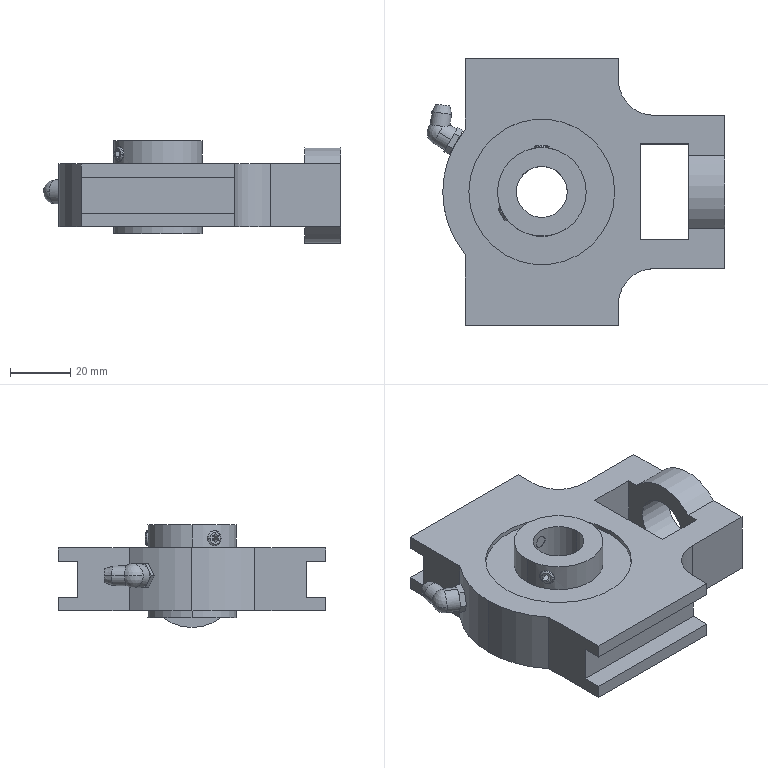Part | STEP file | UCT203 | 2 solids | 99 faces | box 99.208 x 89 x 34.3 mm | volume 116235 mm3 | plane 59 | cylinder 32 | cone 6 | sphere 2 | commonest cylinder face diameters 4.019 x5 5 x4 29.6 x4 48.6 x4 32 x3 6.6 x2